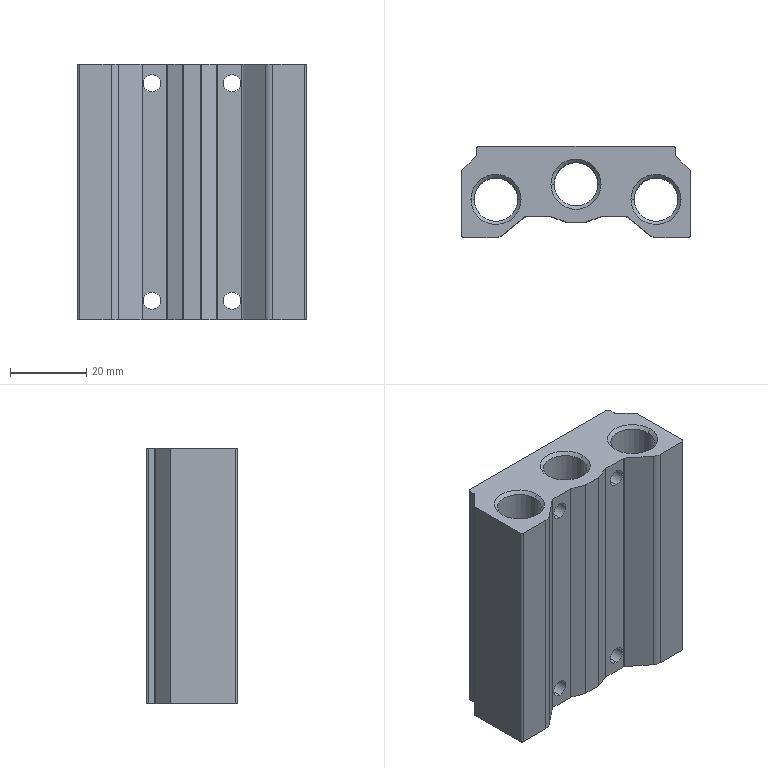Part | SolidWorks | features BaseBody 1 | 1 solid | 98 faces | box 60 x 24 x 67 mm | volume 58558 mm3 | cylinder 48 | cone 28 | plane 22 | commonest cylinder face diameters 1 x12 2.459 x8 4.5 x8 6.5 x8 11.445 x6 10.2 x4